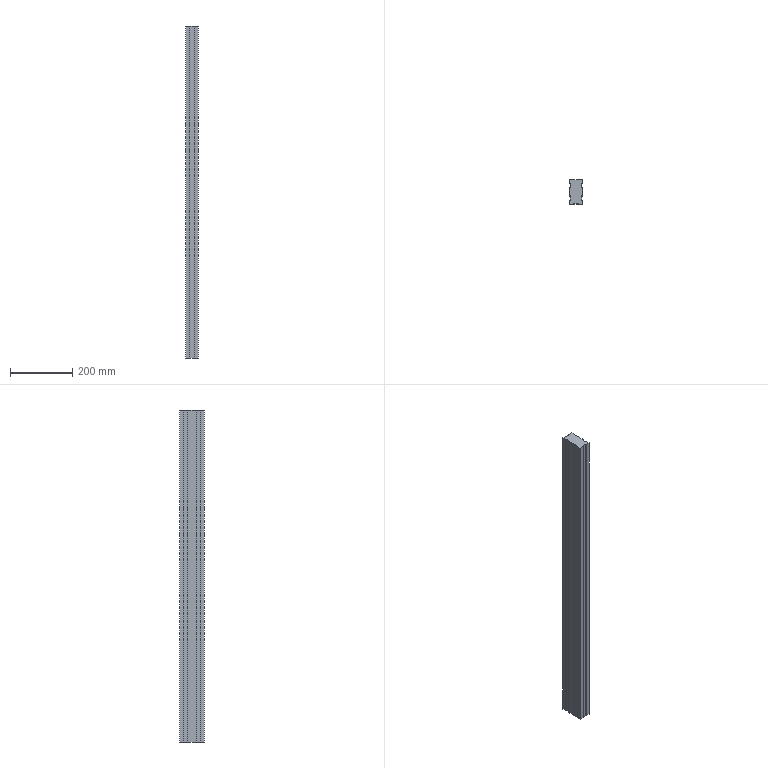Part | STEP file | xingcai40x80x1070 | 1 solid | 30 faces | box 40 x 80 x 1070 mm | volume 3244240 mm3 | plane 30